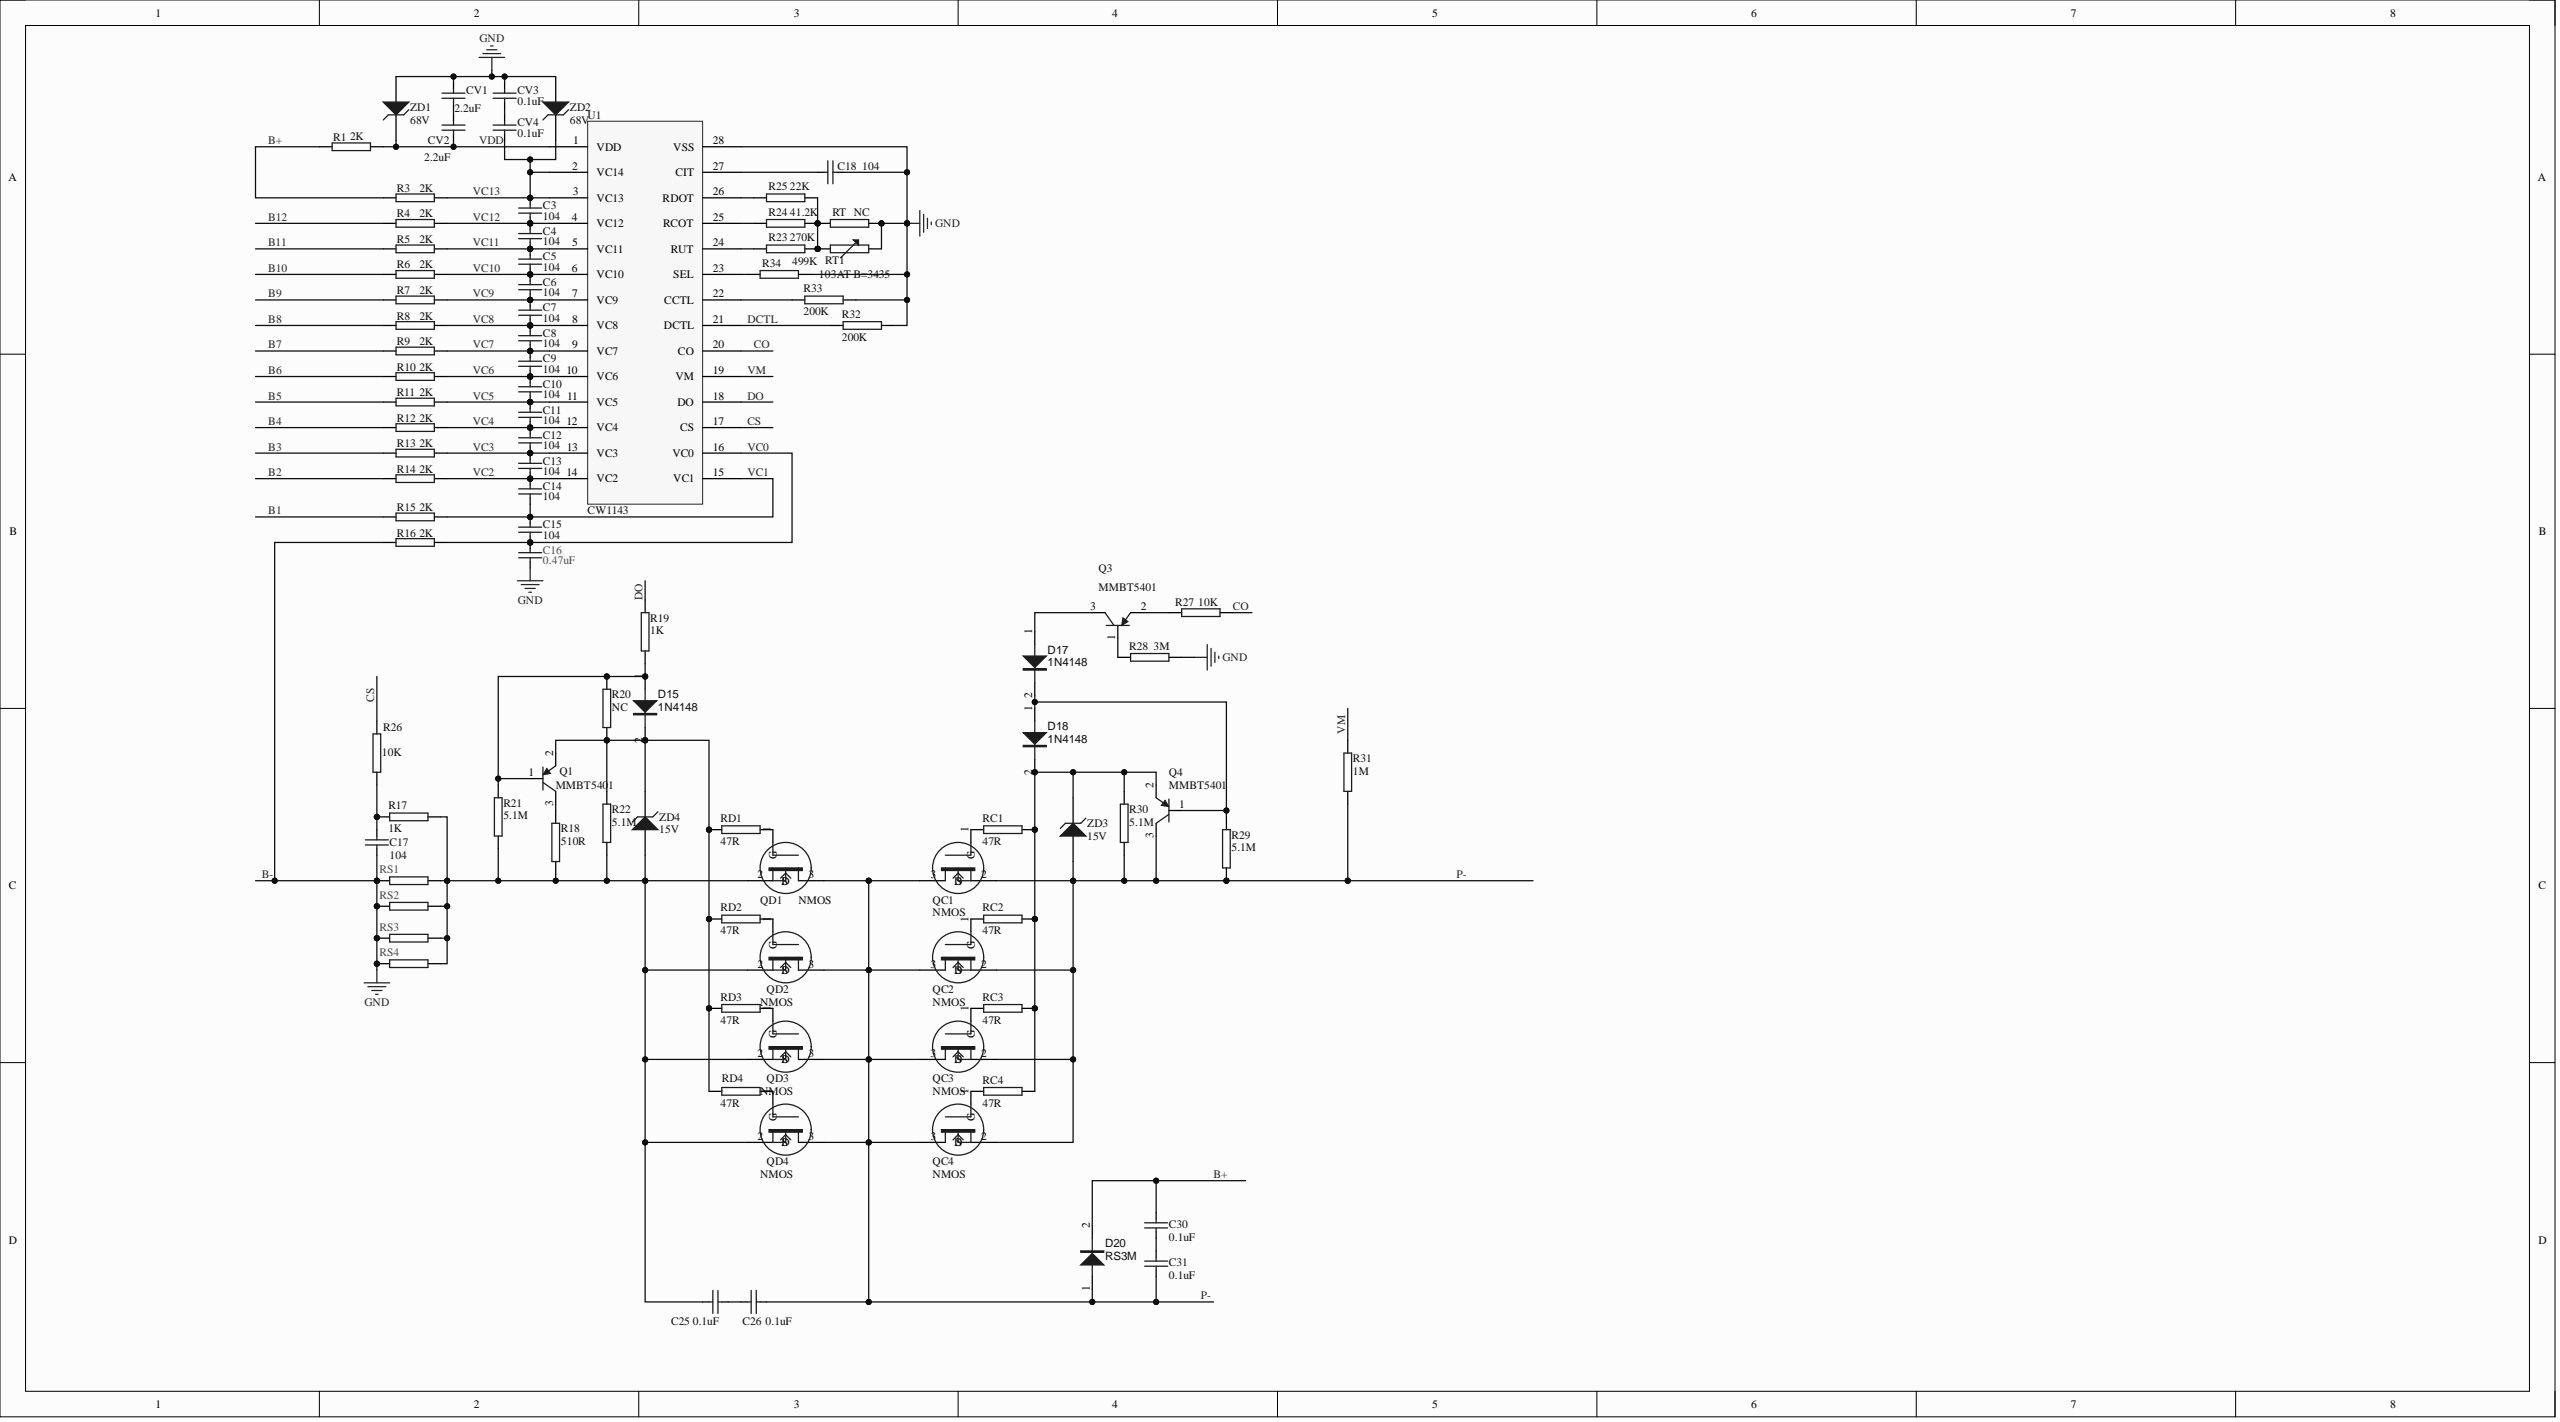Circuit board | Altium Designer | 91 parts | 52 nets
Bill of materials:
Comment,Description,Designator,Footprint,LibRef,Quantity
"104","","C3, C4, C5, C6, C7, C8, C9, C10, C11, C12, C13, C14, C15, C17, C18","CAP0603","CAP","15"
"0.47uF","","C16","CAP0603","CAP","1"
"0.1uF","","C25, C26, C30, C31, CV3, CV4","CAP0603","CAP","6"
"2.2uF","","CV1, CV2","CAP0805","CAP","2"
"1N4148","DIODE","D15, D17, D18","SOD323","DIODE","3"
"RS3M","DIODE","D20","SMC","DIODE","1"
"MMBT5401","PNP Bipolar Transistor","Q1, Q3, Q4","SOT-23-3","PNP","3"
"NMOS","","QC1, QC2, QC3, QC4, QD1, QD2, QD3, QD4","TOLL_123","NMOS","8"
"2K","","R1","RES0805","RES","1"
"2K","","R3, R4, R5, R6, R7, R8, R9, R10, R11, R12, R13, R14, R15, R16","RES0603","RES","14"
"1K","","R17, R19","RES0603","RES","2"
"510R","","R18","RES0603","RES","1"
"NC","","R20, RT","RES0603","RES","2"
"5.1M","","R21, R22, R29, R30","RES0603","RES","4"
"270K","","R23","RES0603","RES","1"
"41.2K","","R24","RES0603","RES","1"
"22K","","R25","RES0603","RES","1"
"10K","","R26, R27","RES0603","RES","2"
"3M","","R28","RES0603","RES","1"
"1M","","R31","RES0603","RES","1"
"200K","","R32, R33","RES0603","RES","2"
"499K","","R34","RES0603","RES","1"
"47R","","RC1, RC2, RC3, RC4, RD1, RD2, RD3, RD4","RES0603","RES","8"
"","","RS1, RS2, RS3, RS4","2512","RES","4"
"103AT B=3435","","RT1","WK","RT1","1"
"CW1143","","U1","SSOP-28-0.635","CW1143","1"
"68V","Zener Diode","ZD1, ZD2","SOD123","D Zener","2"
"15V","Zener Diode","ZD3, ZD4","SOD323","D Zener","2"
Netlist (Protel format):
[
C3
CAP0603
104



]
[
C4
CAP0603
104



]
[
C5
CAP0603
104



]
[
C6
CAP0603
104



]
[
C7
CAP0603
104



]
[
C8
CAP0603
104



]
[
C9
CAP0603
104



]
[
C10
CAP0603
104



]
[
C11
CAP0603
104



]
[
C12
CAP0603
104



]
[
C13
CAP0603
104



]
[
C14
CAP0603
104



]
[
C15
CAP0603
104



]
[
C16
CAP0603
0.47uF



]
[
C17
CAP0603
104



]
[
C18
CAP0603
104



]
[
C25
CAP0603
0.1uF



]
[
C26
CAP0603
0.1uF



]
[
C30
CAP0603
0.1uF



]
[
C31
CAP0603
0.1uF



]
[
CV1
CAP0805
2.2uF



]
[
CV2
CAP0805
2.2uF



]
[
CV3
CAP0603
0.1uF



]
[
CV4
CAP0603
0.1uF



]
[
D15
SOD323
1N4148



]
[
D17
SOD323
1N4148



]
[
D18
SOD323
1N4148



]
[
D20
SMC
RS3M



]
[
Q1
SOT-23-3
MMBT5401



]
[
Q3
SOT-23-3
MMBT5401



]
[
Q4
SOT-23-3
MMBT5401



]
[
QC1
TOLL_123
NMOS



]
[
QC2
TOLL_123
NMOS



]
[
QC3
TOLL_123
NMOS



]
[
QC4
TOLL_123
NMOS



]
[
QD1
TOLL_123
NMOS



]
[
QD2
TOLL_123
NMOS



]
[
QD3
TOLL_123
NMOS



]
[
QD4
TOLL_123
NMOS



]
[
R1
RES0805
2K



]
[
R3
RES0603
2K



]
[
R4
RES0603
2K



]
[
R5
RES0603
2K



]
[
R6
RES0603
2K



]
[
R7
RES0603
2K



]
[
R8
RES0603
2K



]
[
R9
RES0603
2K



]
[
R10
RES0603
2K



]
[
R11
RES0603
2K



]
[
R12
RES0603
2K



]
[
R13
RES0603
2K



]
[
R14
RES0603
2K



]
[
R15
RES0603
2K



]
[
R16
RES0603
2K



]
[
R17
RES0603
1K



]
[
R18
RES0603
510R



]
[
R19
RES0603
1K



]
[
R20
RES0603
NC



]
[
R21
RES0603
5.1M



]
[
R22
RES0603
5.1M



]
[
R23
RES0603
270K



]
[
R24
RES0603
41.2K



]
[
R25
RES0603
22K



]
[
R26
RES0603
10K



]
[
R27
RES0603
10K



]
[
R28
RES0603
3M



]
[
R29
RES0603
5.1M



]
[
R30
RES0603
5.1M



]
[
R31
RES0603
1M



]
[
R32
RES0603
200K



]
[
R33
RES0603
200K



]
[
R34
RES0603
499K



]
[
RC1
RES0603
47R



]
[
RC2
RES0603
47R



]
[
RC3
RES0603
47R



]
[
RC4
RES0603
47R



]
[
RD1
RES0603
47R



]
[
RD2
RES0603
47R



]
[
RD3
RES0603
47R



]
[
RD4
RES0603
47R



]
[
RS1
2512




]
[
RS2
2512




]
[
RS3
2512




]
[
RS4
2512




]
[
RT
RES0603
NC



]
[
RT1
WK
103AT B=3435



]
[
U1
SSOP-28-0.635
CW1143



]
[
ZD1
SOD123
68V



]
[
ZD2
SOD123
68V



]
[
ZD3
SOD323
15V



]
[
ZD4
SOD323
15V



]
(
VM
R31-1
U1-19
)
(
VDD
CV2-2
R1-2
U1-1
ZD1-2
)
(
VC13
C3-1
CV4-2
R3-2
U1-2
U1-3
ZD2-2
)
(
VC12
C3-2
C4-1
R4-2
U1-4
)
(
VC11
C4-2
C5-1
R5-2
U1-5
)
(
VC10
C5-2
C6-1
R6-2
U1-6
)
(
VC9
C6-2
C7-1
R7-2
U1-7
)
(
VC8
C7-2
C8-1
R8-2
U1-8
)
(
VC7
C8-2
C9-1
R9-2
U1-9
)
(
VC6
C9-2
C10-1
R10-2
U1-10
)
(
VC5
C10-2
C11-1
R11-2
U1-11
)
(
VC4
C11-2
C12-1
R12-2
U1-12
)
(
VC3
C12-2
C13-1
R13-2
U1-13
)
(
VC2
C13-2
C14-1
R14-2
U1-14
)
(
VC1
C14-2
C15-1
R15-2
U1-15
)
(
VC0
C15-2
C16-1
R16-2
U1-16
)
(
P-
C26-2
C31-1
D20-1
Q4-3
QC1-2
QC1-3
QC2-2
QC2-3
QC3-2
QC3-3
QC4-2
QC4-3
QD1-3
QD2-3
QD3-3
QD4-3
R29-2
R30-2
R31-2
ZD3-1
)
(
NetR34_1
R34-1
U1-23
)
(
NetR33_1
R33-1
U1-22
)
(
NetR25_1
R25-1
U1-26
)
(
NetR24_1
R24-1
U1-25
)
(
NetR23_2
R23-2
R24-2
R25-2
RT-1
RT1-1
)
(
NetR23_1
R23-1
U1-24
)
(
NetQD4_1
QD4-1
RD4-2
)
(
NetQD3_1
QD3-1
RD3-2
)
(
NetQD2_1
QD2-1
RD2-2
)
(
NetQD1_1
QD1-1
RD1-2
)
(
NetQC4_1
QC4-1
RC4-2
)
(
NetQC3_1
QC3-1
RC3-2
)
(
NetQC2_1
QC2-1
RC2-2
)
(
NetQC1_1
QC1-1
RC1-2
)
(
NetQ3_2
Q3-2
R27-1
)
(
NetQ3_1
Q3-1
R28-2
)
(
NetQ1_3
Q1-3
R18-1
)
(
NetD18_2
D18-2
Q4-2
R30-1
RC1-1
RC2-1
RC3-1
RC4-1
ZD3-2
)
(
NetD17_2
D17-2
D18-1
Q4-1
R29-1
)
(
NetD17_1
D17-1
Q3-3
)
(
NetD15_2
D15-2
Q1-2
R20-2
R22-1
RD1-1
RD2-1
RD3-1
RD4-1
ZD4-2
)
(
NetD15_1
D15-1
Q1-1
R19-2
R20-1
R21-1
)
(
NetCV3_2
CV3-2
CV4-1
)
(
NetCV1_2
CV1-2
CV2-1
)
(
NetC30_1
C30-1
C31-2
)
(
NetC25_2
C25-2
C26-1
)
(
NetC25_1
C25-1
QD1-2
QD2-2
QD3-2
QD4-2
R17-2
R18-2
R21-2
R22-2
RS1-1
RS2-1
RS3-1
RS4-1
ZD4-1
)
(
NetC18_1
C18-1
U1-27
)
(
NetC17_1
C17-1
R17-1
R26-1
)
(
DO
R19-1
U1-18
)
(
DCTL
R32-1
U1-21
)
(
CS
R26-2
U1-17
)
(
CO
R27-2
U1-20
)
(
B-
C16-2
C17-2
C18-2
CV1-1
CV3-1
R16-1
R28-1
R32-2
R33-2
R34-2
RS1-2
RS2-2
RS3-2
RS4-2
RT-2
RT1-2
U1-28
ZD1-1
ZD2-1
)
(
B+
C30-2
D20-2
R1-1
R3-1
)